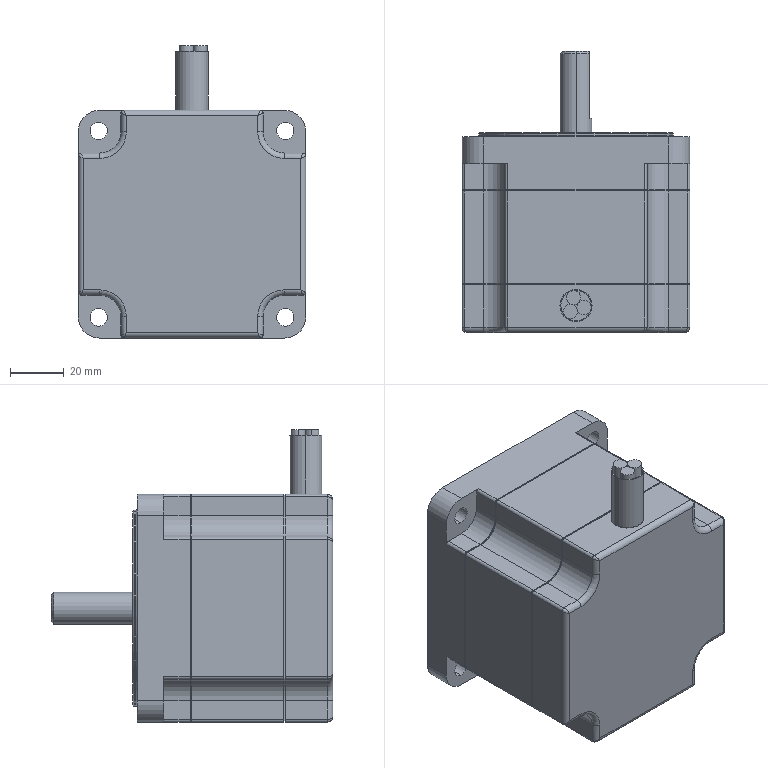Part | SolidWorks | features ICE 14, Fillet 8, Chamfer 3, CirPattern 2, Extrusion 1, MirrorPattern 1 | 4 solids | 191 faces | box 85 x 105 x 109 mm | volume 475306 mm3 | cylinder 86 | plane 84 | torus 10 | spline 8 | cone 3 | commonest cylinder face diameters 2 x24 16 x16 4 x12 6.5 x8 16.6 x8 5.291 x6